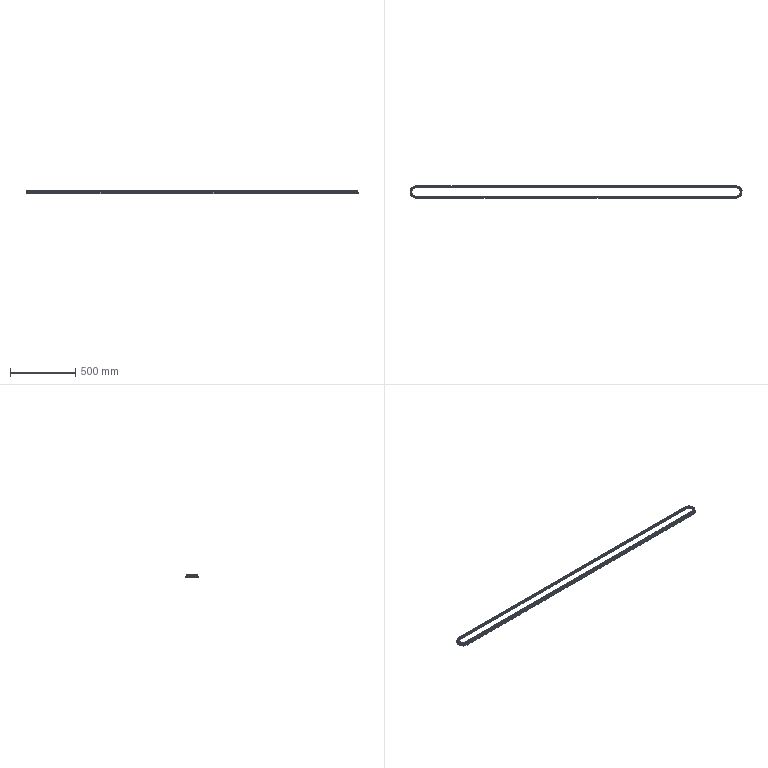Part | SolidWorks | features ReferencePattern 402, LocalChainPattern 1 | 606 solids | 14544 faces | volume 534431 mm3 | cylinder 9898 | plane 4646 | commonest cylinder face diameters 3.98 x3232 10.41 x1616 20 x1414 12.07 x1212 3.4 x808 7.95 x808